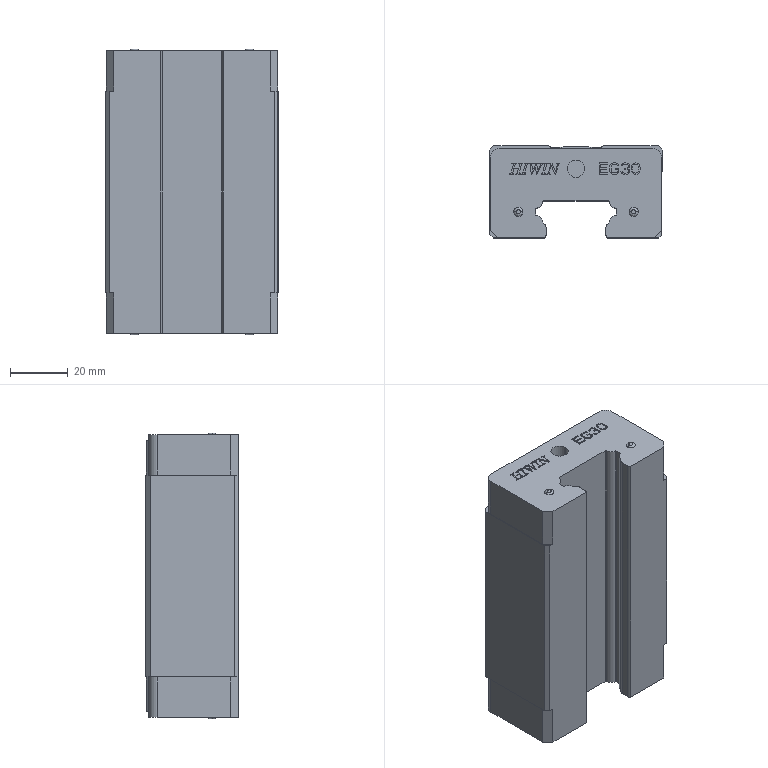Part | STEP file | HIWIN slider EGH30CA | 1 solid | 410 faces | box 60 x 32 x 99.1 mm | volume 151904 mm3 | plane 300 | spline 60 | cylinder 34 | other 8 | cone 8 | commonest cylinder face diameters 6 x8 8 x8 0.6 x4 3.2 x4 5.1 x4 7.3 x4